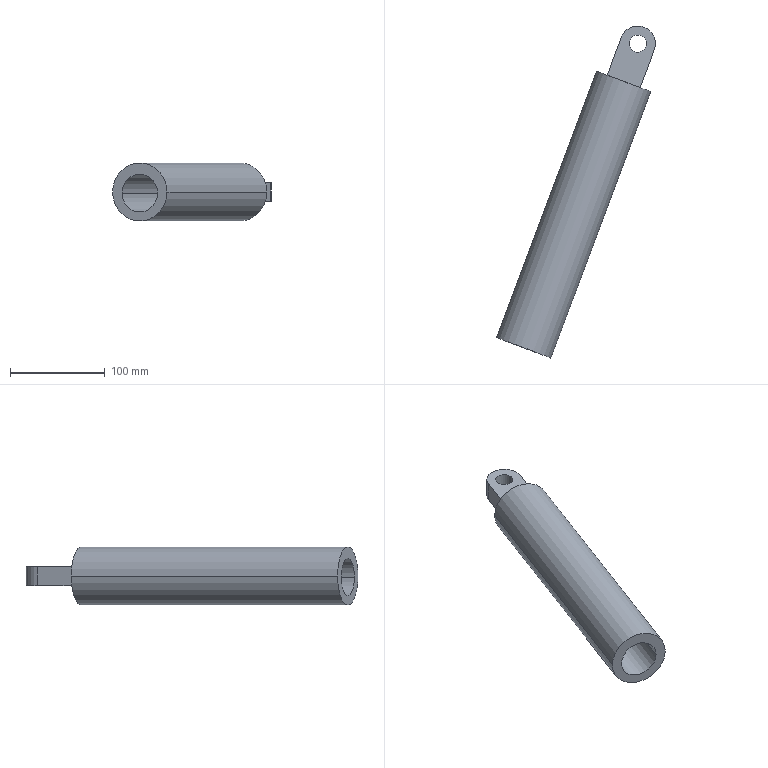Part | SolidWorks | features ICE 2, Extrusion 1 | 1 solid | 15 faces | box 167.58 x 350.157 x 61.299 mm | volume 596100 mm3 | cylinder 8 | plane 7 | commonest cylinder face diameters 18 x2 37.198 x2 40 x2 61.299 x2
STEP:
#1=CARTESIAN_POINT('',(719.886,421.182,2333.834));
#2=VERTEX_POINT('',#1);
#3=CARTESIAN_POINT('',(757.34,407.139,2333.834));
#4=VERTEX_POINT('',#3);
#5=CARTESIAN_POINT('',(738.613,414.16,2333.834));
#6=DIRECTION('',(-0.3511,-0.9363,0.));
#7=DIRECTION('',(0.9363,-0.3511,0.));
#8=AXIS2_PLACEMENT_3D('',#5,#6,#7);
#9=CIRCLE('',#8,20.);
#10=EDGE_CURVE('',#2,#4,#9,.T.);
#11=ORIENTED_EDGE('',*,*,#10,.F.);
#12=CARTESIAN_POINT('',(628.605,177.732,2333.834));
#13=VERTEX_POINT('',#12);
#14=CARTESIAN_POINT('',(719.886,421.182,2333.834));
#15=DIRECTION('',(-0.3511,-0.9363,0.));
#16=VECTOR('',#15,1000.);
#17=LINE('',#14,#16);
#18=EDGE_CURVE('',#2,#13,#17,.T.);
#19=ORIENTED_EDGE('',*,*,#18,.T.);
#20=CARTESIAN_POINT('',(666.059,163.689,2333.834));
#21=VERTEX_POINT('',#20);
#22=CARTESIAN_POINT('',(647.332,170.711,2333.834));
#23=DIRECTION('',(-0.3511,-0.9363,0.));
#24=DIRECTION('',(0.9363,-0.3511,0.));
#25=AXIS2_PLACEMENT_3D('',#22,#23,#24);
#26=CIRCLE('',#25,20.);
#27=EDGE_CURVE('',#13,#21,#26,.T.);
#28=ORIENTED_EDGE('',*,*,#27,.T.);
#29=CARTESIAN_POINT('',(757.34,407.139,2333.834));
#30=DIRECTION('',(-0.3511,-0.9363,0.));
#31=VECTOR('',#30,1000.);
#32=LINE('',#29,#31);
#33=EDGE_CURVE('',#4,#21,#32,.T.);
#34=ORIENTED_EDGE('',*,*,#33,.F.);
#35=EDGE_LOOP('',(#11,#19,#28,#34));
#36=FACE_OUTER_BOUND('',#35,.T.);
#37=CARTESIAN_POINT('',(738.613,414.16,2333.834));
#38=DIRECTION('',(-0.3511,-0.9363,0.));
#39=DIRECTION('',(0.9363,-0.3511,0.));
#40=AXIS2_PLACEMENT_3D('',#37,#38,#39);
#41=CYLINDRICAL_SURFACE('',#40,20.);
#42=ADVANCED_FACE('',(#36),#41,.F.);
#43=CARTESIAN_POINT('',(758.615,491.509,2324.984));
#44=VERTEX_POINT('',#43);
#45=CARTESIAN_POINT('',(776.615,491.509,2324.984));
#46=VERTEX_POINT('',#45);
#47=CARTESIAN_POINT('',(767.615,491.509,2324.984));
#48=DIRECTION('',(0.,0.,1.));
#49=DIRECTION('',(1.,0.,0.));
#50=AXIS2_PLACEMENT_3D('',#47,#48,#49);
#51=CIRCLE('',#50,9.);
#52=EDGE_CURVE('',#44,#46,#51,.T.);
#53=ORIENTED_EDGE('',*,*,#52,.F.);
#54=CARTESIAN_POINT('',(758.615,491.509,2344.984));
#55=VERTEX_POINT('',#54);
#56=CARTESIAN_POINT('',(758.615,491.509,2324.984));
#57=DIRECTION('',(0.,0.,1.));
#58=VECTOR('',#57,1000.);
#59=LINE('',#56,#58);
#60=EDGE_CURVE('',#44,#55,#59,.T.);
#61=ORIENTED_EDGE('',*,*,#60,.T.);
#62=CARTESIAN_POINT('',(776.615,491.509,2344.984));
#63=VERTEX_POINT('',#62);
#64=CARTESIAN_POINT('',(767.615,491.509,2344.984));
#65=DIRECTION('',(0.,0.,1.));
#66=DIRECTION('',(1.,0.,0.));
#67=AXIS2_PLACEMENT_3D('',#64,#65,#66);
#68=CIRCLE('',#67,9.);
#69=EDGE_CURVE('',#55,#63,#68,.T.);
#70=ORIENTED_EDGE('',*,*,#69,.T.);
#71=CARTESIAN_POINT('',(776.615,491.509,2324.984));
#72=DIRECTION('',(0.,0.,1.));
#73=VECTOR('',#72,1000.);
#74=LINE('',#71,#73);
#75=EDGE_CURVE('',#46,#63,#74,.T.);
#76=ORIENTED_EDGE('',*,*,#75,.F.);
#77=EDGE_LOOP('',(#53,#61,#70,#76));
#78=FACE_OUTER_BOUND('',#77,.T.);
#79=CARTESIAN_POINT('',(767.615,491.509,2324.984));
#80=DIRECTION('',(0.,0.,1.));
#81=DIRECTION('',(1.,0.,0.));
#82=AXIS2_PLACEMENT_3D('',#79,#80,#81);
#83=CYLINDRICAL_SURFACE('',#82,9.);
#84=ADVANCED_FACE('',(#78),#83,.F.);
#85=CARTESIAN_POINT('',(785.03,484.979,2324.984));
#86=VERTEX_POINT('',#85);
#87=CARTESIAN_POINT('',(786.214,491.509,2324.984));
#88=VERTEX_POINT('',#87);
#89=CARTESIAN_POINT('',(767.615,491.509,2324.984));
#90=DIRECTION('',(0.,0.,1.));
#91=DIRECTION('',(1.,0.,0.));
#92=AXIS2_PLACEMENT_3D('',#89,#90,#91);
#93=CIRCLE('',#92,18.599);
#94=EDGE_CURVE('',#86,#88,#93,.T.);
#95=ORIENTED_EDGE('',*,*,#94,.T.);
#96=CARTESIAN_POINT('',(786.214,491.509,2344.984));
#97=VERTEX_POINT('',#96);
#98=CARTESIAN_POINT('',(786.214,491.509,2324.984));
#99=DIRECTION('',(0.,0.,1.));
#100=VECTOR('',#99,1000.);
#101=LINE('',#98,#100);
#102=EDGE_CURVE('',#88,#97,#101,.T.);
#103=ORIENTED_EDGE('',*,*,#102,.T.);
#104=CARTESIAN_POINT('',(785.03,484.979,2344.984));
#105=VERTEX_POINT('',#104);
#106=CARTESIAN_POINT('',(767.615,491.509,2344.984));
#107=DIRECTION('',(0.,0.,1.));
#108=DIRECTION('',(1.,0.,0.));
#109=AXIS2_PLACEMENT_3D('',#106,#107,#108);
#110=CIRCLE('',#109,18.599);
#111=EDGE_CURVE('',#105,#97,#110,.T.);
#112=ORIENTED_EDGE('',*,*,#111,.F.);
#113=CARTESIAN_POINT('',(785.03,484.979,2324.984));
#114=DIRECTION('',(0.,0.,1.));
#115=VECTOR('',#114,1000.);
#116=LINE('',#113,#115);
#117=EDGE_CURVE('',#86,#105,#116,.T.);
#118=ORIENTED_EDGE('',*,*,#117,.F.);
#119=EDGE_LOOP('',(#95,#103,#112,#118));
#120=FACE_OUTER_BOUND('',#119,.T.);
#121=CARTESIAN_POINT('',(767.615,491.509,2324.984));
#122=DIRECTION('',(0.,0.,1.));
#123=DIRECTION('',(1.,0.,0.));
#124=AXIS2_PLACEMENT_3D('',#121,#122,#123);
#125=CYLINDRICAL_SURFACE('',#124,18.599);
#126=ADVANCED_FACE('',(#120),#125,.T.);
#127=CARTESIAN_POINT('',(781.355,440.854,2335.07));
#128=VERTEX_POINT('',#127);
#129=CARTESIAN_POINT('',(723.958,462.374,2335.07));
#130=VERTEX_POINT('',#129);
#131=CARTESIAN_POINT('',(752.656,451.614,2335.07));
#132=DIRECTION('',(-0.3511,-0.9363,0.));
#133=DIRECTION('',(0.9363,-0.3511,0.));
#134=AXIS2_PLACEMENT_3D('',#131,#132,#133);
#135=CIRCLE('',#134,30.649);
#136=EDGE_CURVE('',#128,#130,#135,.T.);
#137=ORIENTED_EDGE('',*,*,#136,.T.);
#138=CARTESIAN_POINT('',(618.634,181.471,2335.07));
#139=VERTEX_POINT('',#138);
#140=CARTESIAN_POINT('',(723.958,462.374,2335.07));
#141=DIRECTION('',(-0.3511,-0.9363,0.));
#142=VECTOR('',#141,1000.);
#143=LINE('',#140,#142);
#144=EDGE_CURVE('',#130,#139,#143,.T.);
#145=ORIENTED_EDGE('',*,*,#144,.T.);
#146=CARTESIAN_POINT('',(676.03,159.95,2335.07));
#147=VERTEX_POINT('',#146);
#148=CARTESIAN_POINT('',(647.332,170.711,2335.07));
#149=DIRECTION('',(-0.3511,-0.9363,0.));
#150=DIRECTION('',(0.9363,-0.3511,0.));
#151=AXIS2_PLACEMENT_3D('',#148,#149,#150);
#152=CIRCLE('',#151,30.649);
#153=EDGE_CURVE('',#147,#139,#152,.T.);
#154=ORIENTED_EDGE('',*,*,#153,.F.);
#155=CARTESIAN_POINT('',(781.355,440.854,2335.07));
#156=DIRECTION('',(-0.3511,-0.9363,0.));
#157=VECTOR('',#156,1000.);
#158=LINE('',#155,#157);
#159=EDGE_CURVE('',#128,#147,#158,.T.);
#160=ORIENTED_EDGE('',*,*,#159,.F.);
#161=EDGE_LOOP('',(#137,#145,#154,#160));
#162=FACE_OUTER_BOUND('',#161,.T.);
#163=CARTESIAN_POINT('',(752.656,451.614,2335.07));
#164=DIRECTION('',(-0.3511,-0.9363,0.));
#165=DIRECTION('',(0.9363,-0.3511,0.));
#166=AXIS2_PLACEMENT_3D('',#163,#164,#165);
#167=CYLINDRICAL_SURFACE('',#166,30.649);
#168=ADVANCED_FACE('',(#162),#167,.T.);
#169=ORIENTED_EDGE('',*,*,#136,.F.);
#170=CARTESIAN_POINT('',(752.656,451.614,2335.07));
#171=DIRECTION('',(-0.3511,-0.9363,0.));
#172=DIRECTION('',(0.9363,-0.3511,0.));
#173=AXIS2_PLACEMENT_3D('',#170,#171,#172);
#174=CIRCLE('',#173,30.649);
#175=EDGE_CURVE('',#130,#128,#174,.T.);
#176=ORIENTED_EDGE('',*,*,#175,.F.);
#177=EDGE_LOOP('',(#169,#176));
#178=FACE_OUTER_BOUND('',#177,.T.);
#179=CARTESIAN_POINT('',(735.242,458.144,2344.984));
#180=VERTEX_POINT('',#179);
#181=CARTESIAN_POINT('',(770.071,445.084,2344.984));
#182=VERTEX_POINT('',#181);
#183=CARTESIAN_POINT('',(735.242,458.144,2344.984));
#184=DIRECTION('',(0.9363,-0.3511,0.));
#185=VECTOR('',#184,1000.);
#186=LINE('',#183,#185);
#187=EDGE_CURVE('',#180,#182,#186,.T.);
#188=ORIENTED_EDGE('',*,*,#187,.F.);
#189=CARTESIAN_POINT('',(735.242,458.144,2324.984));
#190=VERTEX_POINT('',#189);
#191=CARTESIAN_POINT('',(735.242,458.144,2324.984));
#192=DIRECTION('',(0.,0.,1.));
#193=VECTOR('',#192,1000.);
#194=LINE('',#191,#193);
#195=EDGE_CURVE('',#190,#180,#194,.T.);
#196=ORIENTED_EDGE('',*,*,#195,.F.);
#197=CARTESIAN_POINT('',(770.071,445.084,2324.984));
#198=VERTEX_POINT('',#197);
#199=CARTESIAN_POINT('',(735.242,458.144,2324.984));
#200=DIRECTION('',(0.9363,-0.3511,0.));
#201=VECTOR('',#200,1000.);
#202=LINE('',#199,#201);
#203=EDGE_CURVE('',#190,#198,#202,.T.);
#204=ORIENTED_EDGE('',*,*,#203,.T.);
#205=CARTESIAN_POINT('',(770.071,445.084,2324.984));
#206=DIRECTION('',(0.,0.,1.));
#207=VECTOR('',#206,1000.);
#208=LINE('',#205,#207);
#209=EDGE_CURVE('',#198,#182,#208,.T.);
#210=ORIENTED_EDGE('',*,*,#209,.T.);
#211=EDGE_LOOP('',(#188,#196,#204,#210));
#212=FACE_BOUND('',#211,.T.);
#213=CARTESIAN_POINT('',(752.656,451.614,2335.07));
#214=DIRECTION('',(-0.3511,-0.9363,0.));
#215=DIRECTION('',(0.9363,-0.3511,0.));
#216=AXIS2_PLACEMENT_3D('',#213,#214,#215);
#217=PLANE('',#216);
#218=ADVANCED_FACE('',(#178,#212),#217,.F.);
#219=ORIENTED_EDGE('',*,*,#144,.F.);
#220=ORIENTED_EDGE('',*,*,#175,.T.);
#221=ORIENTED_EDGE('',*,*,#159,.T.);
#222=CARTESIAN_POINT('',(647.332,170.711,2335.07));
#223=DIRECTION('',(-0.3511,-0.9363,0.));
#224=DIRECTION('',(0.9363,-0.3511,0.));
#225=AXIS2_PLACEMENT_3D('',#222,#223,#224);
#226=CIRCLE('',#225,30.649);
#227=EDGE_CURVE('',#139,#147,#226,.T.);
#228=ORIENTED_EDGE('',*,*,#227,.F.);
#229=EDGE_LOOP('',(#219,#220,#221,#228));
#230=FACE_OUTER_BOUND('',#229,.T.);
#231=CARTESIAN_POINT('',(752.656,451.614,2335.07));
#232=DIRECTION('',(-0.3511,-0.9363,0.));
#233=DIRECTION('',(0.9363,-0.3511,0.));
#234=AXIS2_PLACEMENT_3D('',#231,#232,#233);
#235=CYLINDRICAL_SURFACE('',#234,30.649);
#236=ADVANCED_FACE('',(#230),#235,.T.);
#237=CARTESIAN_POINT('',(647.332,170.711,2333.834));
#238=DIRECTION('',(-0.3511,-0.9363,0.));
#239=DIRECTION('',(0.9363,-0.3511,0.));
#240=AXIS2_PLACEMENT_3D('',#237,#238,#239);
#241=CIRCLE('',#240,20.);
#242=EDGE_CURVE('',#21,#13,#241,.T.);
#243=ORIENTED_EDGE('',*,*,#242,.F.);
#244=ORIENTED_EDGE('',*,*,#27,.F.);
#245=EDGE_LOOP('',(#243,#244));
#246=FACE_BOUND('',#245,.T.);
#247=ORIENTED_EDGE('',*,*,#153,.T.);
#248=ORIENTED_EDGE('',*,*,#227,.T.);
#249=EDGE_LOOP('',(#247,#248));
#250=FACE_OUTER_BOUND('',#249,.T.);
#251=CARTESIAN_POINT('',(647.332,170.711,2335.07));
#252=DIRECTION('',(-0.3511,-0.9363,0.));
#253=DIRECTION('',(0.9363,-0.3511,0.));
#254=AXIS2_PLACEMENT_3D('',#251,#252,#253);
#255=PLANE('',#254);
#256=ADVANCED_FACE('',(#246,#250),#255,.T.);
#257=ORIENTED_EDGE('',*,*,#102,.F.);
#258=CARTESIAN_POINT('',(750.2,498.038,2324.984));
#259=VERTEX_POINT('',#258);
#260=CARTESIAN_POINT('',(767.615,491.509,2324.984));
#261=DIRECTION('',(0.,0.,1.));
#262=DIRECTION('',(1.,0.,0.));
#263=AXIS2_PLACEMENT_3D('',#260,#261,#262);
#264=CIRCLE('',#263,18.599);
#265=EDGE_CURVE('',#88,#259,#264,.T.);
#266=ORIENTED_EDGE('',*,*,#265,.T.);
#267=CARTESIAN_POINT('',(750.2,498.038,2344.984));
#268=VERTEX_POINT('',#267);
#269=CARTESIAN_POINT('',(750.2,498.038,2324.984));
#270=DIRECTION('',(0.,0.,1.));
#271=VECTOR('',#270,1000.);
#272=LINE('',#269,#271);
#273=EDGE_CURVE('',#259,#268,#272,.T.);
#274=ORIENTED_EDGE('',*,*,#273,.T.);
#275=CARTESIAN_POINT('',(767.615,491.509,2344.984));
#276=DIRECTION('',(0.,0.,1.));
#277=DIRECTION('',(1.,0.,0.));
#278=AXIS2_PLACEMENT_3D('',#275,#276,#277);
#279=CIRCLE('',#278,18.599);
#280=EDGE_CURVE('',#97,#268,#279,.T.);
#281=ORIENTED_EDGE('',*,*,#280,.F.);
#282=EDGE_LOOP('',(#257,#266,#274,#281));
#283=FACE_OUTER_BOUND('',#282,.T.);
#284=CARTESIAN_POINT('',(767.615,491.509,2324.984));
#285=DIRECTION('',(0.,0.,1.));
#286=DIRECTION('',(1.,0.,0.));
#287=AXIS2_PLACEMENT_3D('',#284,#285,#286);
#288=CYLINDRICAL_SURFACE('',#287,18.599);
#289=ADVANCED_FACE('',(#283),#288,.T.);
#290=CARTESIAN_POINT('',(770.071,445.084,2344.984));
#291=DIRECTION('',(0.3511,0.9363,0.));
#292=VECTOR('',#291,1000.);
#293=LINE('',#290,#292);
#294=EDGE_CURVE('',#182,#105,#293,.T.);
#295=ORIENTED_EDGE('',*,*,#294,.F.);
#296=ORIENTED_EDGE('',*,*,#209,.F.);
#297=CARTESIAN_POINT('',(770.071,445.084,2324.984));
#298=DIRECTION('',(0.3511,0.9363,0.));
#299=VECTOR('',#298,1000.);
#300=LINE('',#297,#299);
#301=EDGE_CURVE('',#198,#86,#300,.T.);
#302=ORIENTED_EDGE('',*,*,#301,.T.);
#303=ORIENTED_EDGE('',*,*,#117,.T.);
#304=EDGE_LOOP('',(#295,#296,#302,#303));
#305=FACE_OUTER_BOUND('',#304,.T.);
#306=CARTESIAN_POINT('',(770.071,445.084,2324.984));
#307=DIRECTION('',(0.9363,-0.3511,0.));
#308=DIRECTION('',(0.3511,0.9363,0.));
#309=AXIS2_PLACEMENT_3D('',#306,#307,#308);
#310=PLANE('',#309);
#311=ADVANCED_FACE('',(#305),#310,.T.);
#312=CARTESIAN_POINT('',(750.2,498.038,2344.984));
#313=DIRECTION('',(-0.3511,-0.9363,0.));
#314=VECTOR('',#313,1000.);
#315=LINE('',#312,#314);
#316=EDGE_CURVE('',#268,#180,#315,.T.);
#317=ORIENTED_EDGE('',*,*,#316,.F.);
#318=ORIENTED_EDGE('',*,*,#273,.F.);
#319=CARTESIAN_POINT('',(750.2,498.038,2324.984));
#320=DIRECTION('',(-0.3511,-0.9363,0.));
#321=VECTOR('',#320,1000.);
#322=LINE('',#319,#321);
#323=EDGE_CURVE('',#259,#190,#322,.T.);
#324=ORIENTED_EDGE('',*,*,#323,.T.);
#325=ORIENTED_EDGE('',*,*,#195,.T.);
#326=EDGE_LOOP('',(#317,#318,#324,#325));
#327=FACE_OUTER_BOUND('',#326,.T.);
#328=CARTESIAN_POINT('',(750.2,498.038,2324.984));
#329=DIRECTION('',(-0.9363,0.3511,0.));
#330=DIRECTION('',(-0.3511,-0.9363,0.));
#331=AXIS2_PLACEMENT_3D('',#328,#329,#330);
#332=PLANE('',#331);
#333=ADVANCED_FACE('',(#327),#332,.T.);
#334=CARTESIAN_POINT('',(767.615,491.509,2324.984));
#335=DIRECTION('',(0.,0.,1.));
#336=DIRECTION('',(1.,0.,0.));
#337=AXIS2_PLACEMENT_3D('',#334,#335,#336);
#338=CIRCLE('',#337,9.);
#339=EDGE_CURVE('',#46,#44,#338,.T.);
#340=ORIENTED_EDGE('',*,*,#339,.T.);
#341=ORIENTED_EDGE('',*,*,#52,.T.);
#342=EDGE_LOOP('',(#340,#341));
#343=FACE_BOUND('',#342,.T.);
#344=ORIENTED_EDGE('',*,*,#94,.F.);
#345=ORIENTED_EDGE('',*,*,#301,.F.);
#346=ORIENTED_EDGE('',*,*,#203,.F.);
#347=ORIENTED_EDGE('',*,*,#323,.F.);
#348=ORIENTED_EDGE('',*,*,#265,.F.);
#349=EDGE_LOOP('',(#344,#345,#346,#347,#348));
#350=FACE_OUTER_BOUND('',#349,.T.);
#351=CARTESIAN_POINT('',(767.615,491.509,2324.984));
#352=DIRECTION('',(0.,0.,1.));
#353=DIRECTION('',(1.,0.,0.));
#354=AXIS2_PLACEMENT_3D('',#351,#352,#353);
#355=PLANE('',#354);
#356=ADVANCED_FACE('',(#343,#350),#355,.F.);
#357=CARTESIAN_POINT('',(767.615,491.509,2344.984));
#358=DIRECTION('',(0.,0.,1.));
#359=DIRECTION('',(1.,0.,0.));
#360=AXIS2_PLACEMENT_3D('',#357,#358,#359);
#361=CIRCLE('',#360,9.);
#362=EDGE_CURVE('',#63,#55,#361,.T.);
#363=ORIENTED_EDGE('',*,*,#362,.F.);
#364=ORIENTED_EDGE('',*,*,#69,.F.);
#365=EDGE_LOOP('',(#363,#364));
#366=FACE_BOUND('',#365,.T.);
#367=ORIENTED_EDGE('',*,*,#111,.T.);
#368=ORIENTED_EDGE('',*,*,#280,.T.);
#369=ORIENTED_EDGE('',*,*,#316,.T.);
#370=ORIENTED_EDGE('',*,*,#187,.T.);
#371=ORIENTED_EDGE('',*,*,#294,.T.);
#372=EDGE_LOOP('',(#367,#368,#369,#370,#371));
#373=FACE_OUTER_BOUND('',#372,.T.);
#374=CARTESIAN_POINT('',(767.615,491.509,2344.984));
#375=DIRECTION('',(0.,0.,1.));
#376=DIRECTION('',(1.,0.,0.));
#377=AXIS2_PLACEMENT_3D('',#374,#375,#376);
#378=PLANE('',#377);
#379=ADVANCED_FACE('',(#366,#373),#378,.T.);
#380=ORIENTED_EDGE('',*,*,#60,.F.);
#381=ORIENTED_EDGE('',*,*,#339,.F.);
#382=ORIENTED_EDGE('',*,*,#75,.T.);
#383=ORIENTED_EDGE('',*,*,#362,.T.);
#384=EDGE_LOOP('',(#380,#381,#382,#383));
#385=FACE_OUTER_BOUND('',#384,.T.);
#386=CARTESIAN_POINT('',(767.615,491.509,2324.984));
#387=DIRECTION('',(0.,0.,1.));
#388=DIRECTION('',(1.,0.,0.));
#389=AXIS2_PLACEMENT_3D('',#386,#387,#388);
#390=CYLINDRICAL_SURFACE('',#389,9.);
#391=ADVANCED_FACE('',(#385),#390,.F.);
#392=ORIENTED_EDGE('',*,*,#18,.F.);
#393=CARTESIAN_POINT('',(738.613,414.16,2333.834));
#394=DIRECTION('',(-0.3511,-0.9363,0.));
#395=DIRECTION('',(0.9363,-0.3511,0.));
#396=AXIS2_PLACEMENT_3D('',#393,#394,#395);
#397=CIRCLE('',#396,20.);
#398=EDGE_CURVE('',#4,#2,#397,.T.);
#399=ORIENTED_EDGE('',*,*,#398,.F.);
#400=ORIENTED_EDGE('',*,*,#33,.T.);
#401=ORIENTED_EDGE('',*,*,#242,.T.);
#402=EDGE_LOOP('',(#392,#399,#400,#401));
#403=FACE_OUTER_BOUND('',#402,.T.);
#404=CARTESIAN_POINT('',(738.613,414.16,2333.834));
#405=DIRECTION('',(-0.3511,-0.9363,0.));
#406=DIRECTION('',(0.9363,-0.3511,0.));
#407=AXIS2_PLACEMENT_3D('',#404,#405,#406);
#408=CYLINDRICAL_SURFACE('',#407,20.);
#409=ADVANCED_FACE('',(#403),#408,.F.);
#410=ORIENTED_EDGE('',*,*,#398,.T.);
#411=ORIENTED_EDGE('',*,*,#10,.T.);
#412=EDGE_LOOP('',(#410,#411));
#413=FACE_OUTER_BOUND('',#412,.T.);
#414=CARTESIAN_POINT('',(738.613,414.16,2333.834));
#415=DIRECTION('',(-0.3511,-0.9363,0.));
#416=DIRECTION('',(0.9363,-0.3511,0.));
#417=AXIS2_PLACEMENT_3D('',#414,#415,#416);
#418=PLANE('',#417);
#419=ADVANCED_FACE('',(#413),#418,.T.);
#420=CLOSED_SHELL('',(#42,#84,#126,#168,#218,#236,#256,#289,#311,#333,#356,#379,#391,#409,#419));
#421=MANIFOLD_SOLID_BREP('',#420);
#422=CARTESIAN_POINT('',(0.,0.,0.));
#423=DIRECTION('',(0.,0.,1.));
#424=DIRECTION('',(1.,0.,0.));
#425=AXIS2_PLACEMENT_3D('',#422,#423,#424);
#426=(LENGTH_UNIT()NAMED_UNIT(*)SI_UNIT(.MILLI.,.METRE.));
#427=UNCERTAINTY_MEASURE_WITH_UNIT(LENGTH_MEASURE(0.00001),#426,'','');
#428=(NAMED_UNIT(*)PLANE_ANGLE_UNIT()SI_UNIT($,.RADIAN.));
#429=(NAMED_UNIT(*)SI_UNIT($,.STERADIAN.)SOLID_ANGLE_UNIT());
#430=(GEOMETRIC_REPRESENTATION_CONTEXT(3)GLOBAL_UNCERTAINTY_ASSIGNED_CONTEXT((#427))GLOBAL_UNIT_ASSIGNED_CONTEXT((#426,#428,#429))REPRESENTATION_CONTEXT('',''));
#431=ADVANCED_BREP_SHAPE_REPRESENTATION('',(#421,#425),#430);